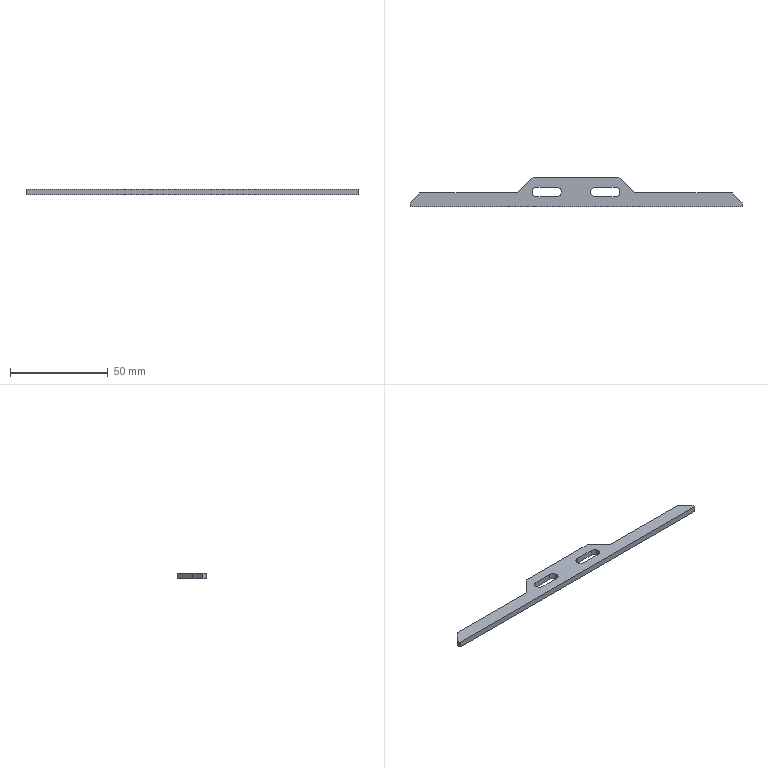Part | STEP file | GLSJ-10-17_default | 1 solid | 22 faces | box 170 x 15 x 3 mm | volume 4325 mm3 | plane 16 | cylinder 6 | commonest cylinder face diameters 5 x6